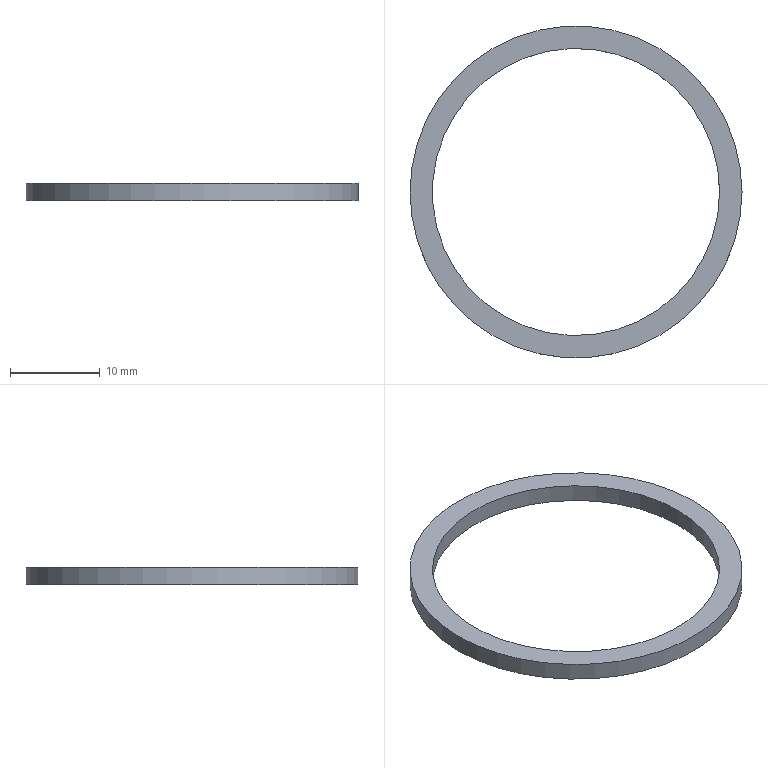Part | NX | features BREP 1 | 1 solid | 4 faces | box 37 x 37 x 2 mm | volume 541.925 mm3 | cylinder 2 | plane 2 | commonest cylinder face diameters 32 x1 37 x1
STEP:
#1=CARTESIAN_POINT('',(16.,0.,0.));
#2=VERTEX_POINT('',#1);
#3=CARTESIAN_POINT('',(0.,0.,0.));
#4=DIRECTION('',(0.,0.,1.));
#5=DIRECTION('',(1.,0.,0.));
#6=AXIS2_PLACEMENT_3D('',#3,#4,#5);
#7=CIRCLE('',#6,16.);
#8=EDGE_CURVE('',#2,#2,#7,.T.);
#9=ORIENTED_EDGE('',*,*,#8,.F.);
#10=EDGE_LOOP('',(#9));
#11=FACE_BOUND('',#10,.T.);
#12=CARTESIAN_POINT('',(16.,0.,2.));
#13=VERTEX_POINT('',#12);
#14=CARTESIAN_POINT('',(0.,0.,2.));
#15=DIRECTION('',(0.,0.,1.));
#16=DIRECTION('',(1.,0.,0.));
#17=AXIS2_PLACEMENT_3D('',#14,#15,#16);
#18=CIRCLE('',#17,16.);
#19=EDGE_CURVE('',#13,#13,#18,.T.);
#20=ORIENTED_EDGE('',*,*,#19,.T.);
#21=EDGE_LOOP('',(#20));
#22=FACE_BOUND('',#21,.T.);
#23=CARTESIAN_POINT('',(0.,0.,2.));
#24=DIRECTION('',(0.,0.,-1.));
#25=DIRECTION('',(-1.,0.,0.));
#26=AXIS2_PLACEMENT_3D('',#23,#24,#25);
#27=CYLINDRICAL_SURFACE('',#26,16.);
#28=ADVANCED_FACE('',(#11,#22),#27,.F.);
#29=CARTESIAN_POINT('',(18.5,0.,0.));
#30=VERTEX_POINT('',#29);
#31=CARTESIAN_POINT('',(0.,0.,0.));
#32=DIRECTION('',(0.,0.,1.));
#33=DIRECTION('',(1.,0.,0.));
#34=AXIS2_PLACEMENT_3D('',#31,#32,#33);
#35=CIRCLE('',#34,18.5);
#36=EDGE_CURVE('',#30,#30,#35,.T.);
#37=ORIENTED_EDGE('',*,*,#36,.T.);
#38=EDGE_LOOP('',(#37));
#39=FACE_BOUND('',#38,.T.);
#40=CARTESIAN_POINT('',(18.5,0.,2.));
#41=VERTEX_POINT('',#40);
#42=CARTESIAN_POINT('',(0.,0.,2.));
#43=DIRECTION('',(0.,0.,1.));
#44=DIRECTION('',(1.,0.,0.));
#45=AXIS2_PLACEMENT_3D('',#42,#43,#44);
#46=CIRCLE('',#45,18.5);
#47=EDGE_CURVE('',#41,#41,#46,.T.);
#48=ORIENTED_EDGE('',*,*,#47,.F.);
#49=EDGE_LOOP('',(#48));
#50=FACE_BOUND('',#49,.T.);
#51=CARTESIAN_POINT('',(0.,0.,2.));
#52=DIRECTION('',(0.,0.,-1.));
#53=DIRECTION('',(-1.,0.,0.));
#54=AXIS2_PLACEMENT_3D('',#51,#52,#53);
#55=CYLINDRICAL_SURFACE('',#54,18.5);
#56=ADVANCED_FACE('',(#39,#50),#55,.T.);
#57=ORIENTED_EDGE('',*,*,#47,.T.);
#58=EDGE_LOOP('',(#57));
#59=FACE_BOUND('',#58,.T.);
#60=ORIENTED_EDGE('',*,*,#19,.F.);
#61=EDGE_LOOP('',(#60));
#62=FACE_BOUND('',#61,.T.);
#63=CARTESIAN_POINT('',(0.,0.,2.));
#64=DIRECTION('',(0.,0.,1.));
#65=DIRECTION('',(1.,0.,0.));
#66=AXIS2_PLACEMENT_3D('',#63,#64,#65);
#67=PLANE('',#66);
#68=ADVANCED_FACE('',(#59,#62),#67,.T.);
#69=ORIENTED_EDGE('',*,*,#36,.F.);
#70=EDGE_LOOP('',(#69));
#71=FACE_BOUND('',#70,.T.);
#72=ORIENTED_EDGE('',*,*,#8,.T.);
#73=EDGE_LOOP('',(#72));
#74=FACE_BOUND('',#73,.T.);
#75=CARTESIAN_POINT('',(0.,0.,0.));
#76=DIRECTION('',(0.,0.,1.));
#77=DIRECTION('',(1.,0.,0.));
#78=AXIS2_PLACEMENT_3D('',#75,#76,#77);
#79=PLANE('',#78);
#80=ADVANCED_FACE('',(#71,#74),#79,.F.);
#81=CLOSED_SHELL('',(#28,#56,#68,#80));
#82=MANIFOLD_SOLID_BREP('',#81);
#83=(LENGTH_UNIT()NAMED_UNIT(*)SI_UNIT(.MILLI.,.METRE.));
#84=UNCERTAINTY_MEASURE_WITH_UNIT(LENGTH_MEASURE(0.00001),#83,'','');
#85=(NAMED_UNIT(*)PLANE_ANGLE_UNIT()SI_UNIT($,.RADIAN.));
#86=(NAMED_UNIT(*)SI_UNIT($,.STERADIAN.)SOLID_ANGLE_UNIT());
#87=(GEOMETRIC_REPRESENTATION_CONTEXT(3)GLOBAL_UNCERTAINTY_ASSIGNED_CONTEXT((#84))GLOBAL_UNIT_ASSIGNED_CONTEXT((#83,#85,#86))REPRESENTATION_CONTEXT('',''));
#88=ADVANCED_BREP_SHAPE_REPRESENTATION('',(#82),#87);